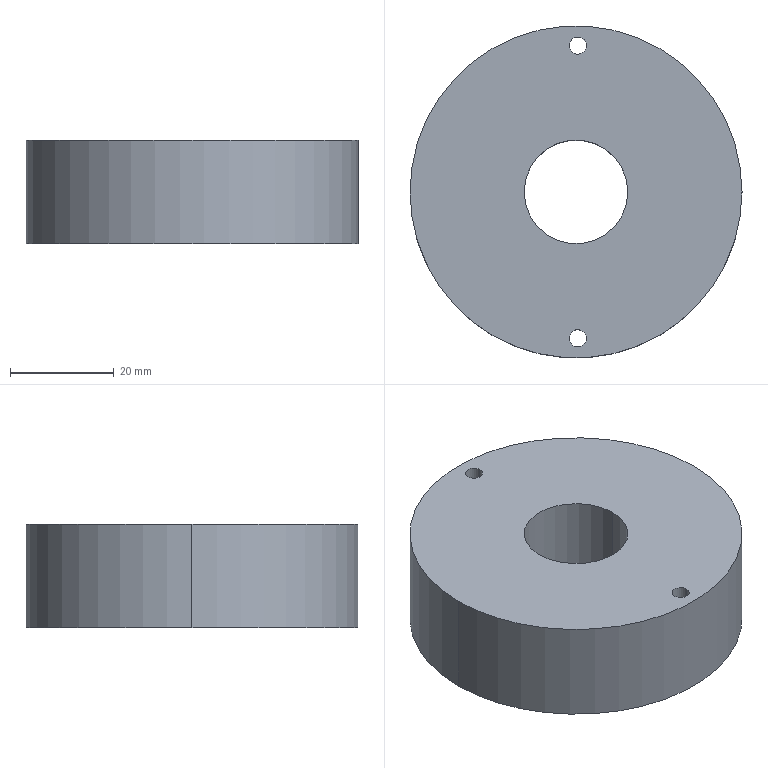Part | SolidWorks | features Extrusion 1, HoleWzd 1 | 1 solid | 10 faces | box 64 x 64 x 20 mm | volume 57715 mm3 | cylinder 8 | plane 2 | commonest cylinder face diameters 3.3 x4 20 x2 64 x2
STEP:
#1=CARTESIAN_POINT('',(-1.65,28.2,20.));
#2=VERTEX_POINT('',#1);
#3=CARTESIAN_POINT('',(1.65,28.2,20.));
#4=VERTEX_POINT('',#3);
#5=CARTESIAN_POINT('',(0.,28.2,20.));
#6=DIRECTION('',(0.,0.,1.));
#7=DIRECTION('',(1.,0.,0.));
#8=AXIS2_PLACEMENT_3D('',#5,#6,#7);
#9=CIRCLE('',#8,1.65);
#10=EDGE_CURVE('',#2,#4,#9,.T.);
#11=ORIENTED_EDGE('',*,*,#10,.T.);
#12=CARTESIAN_POINT('',(1.65,28.2,0.));
#13=VERTEX_POINT('',#12);
#14=CARTESIAN_POINT('',(1.65,28.2,0.));
#15=DIRECTION('',(0.,0.,-1.));
#16=VECTOR('',#15,1000.);
#17=LINE('',#14,#16);
#18=EDGE_CURVE('',#4,#13,#17,.T.);
#19=ORIENTED_EDGE('',*,*,#18,.T.);
#20=CARTESIAN_POINT('',(-1.65,28.2,0.));
#21=VERTEX_POINT('',#20);
#22=CARTESIAN_POINT('',(0.,28.2,0.));
#23=DIRECTION('',(0.,0.,-1.));
#24=DIRECTION('',(-1.,0.,0.));
#25=AXIS2_PLACEMENT_3D('',#22,#23,#24);
#26=CIRCLE('',#25,1.65);
#27=EDGE_CURVE('',#13,#21,#26,.T.);
#28=ORIENTED_EDGE('',*,*,#27,.T.);
#29=CARTESIAN_POINT('',(-1.65,28.2,0.));
#30=DIRECTION('',(0.,0.,-1.));
#31=VECTOR('',#30,1000.);
#32=LINE('',#29,#31);
#33=EDGE_CURVE('',#2,#21,#32,.T.);
#34=ORIENTED_EDGE('',*,*,#33,.F.);
#35=EDGE_LOOP('',(#11,#19,#28,#34));
#36=FACE_OUTER_BOUND('',#35,.T.);
#37=CARTESIAN_POINT('',(0.,28.2,0.));
#38=DIRECTION('',(0.,0.,-1.));
#39=DIRECTION('',(-1.,0.,0.));
#40=AXIS2_PLACEMENT_3D('',#37,#38,#39);
#41=CYLINDRICAL_SURFACE('',#40,1.65);
#42=ADVANCED_FACE('',(#36),#41,.F.);
#43=CARTESIAN_POINT('',(-1.65,-28.2,20.));
#44=VERTEX_POINT('',#43);
#45=CARTESIAN_POINT('',(1.65,-28.2,20.));
#46=VERTEX_POINT('',#45);
#47=CARTESIAN_POINT('',(0.,-28.2,20.));
#48=DIRECTION('',(0.,0.,1.));
#49=DIRECTION('',(1.,0.,0.));
#50=AXIS2_PLACEMENT_3D('',#47,#48,#49);
#51=CIRCLE('',#50,1.65);
#52=EDGE_CURVE('',#44,#46,#51,.T.);
#53=ORIENTED_EDGE('',*,*,#52,.T.);
#54=CARTESIAN_POINT('',(1.65,-28.2,0.));
#55=VERTEX_POINT('',#54);
#56=CARTESIAN_POINT('',(1.65,-28.2,0.));
#57=DIRECTION('',(0.,0.,-1.));
#58=VECTOR('',#57,1000.);
#59=LINE('',#56,#58);
#60=EDGE_CURVE('',#46,#55,#59,.T.);
#61=ORIENTED_EDGE('',*,*,#60,.T.);
#62=CARTESIAN_POINT('',(-1.65,-28.2,0.));
#63=VERTEX_POINT('',#62);
#64=CARTESIAN_POINT('',(0.,-28.2,0.));
#65=DIRECTION('',(0.,0.,-1.));
#66=DIRECTION('',(-1.,0.,0.));
#67=AXIS2_PLACEMENT_3D('',#64,#65,#66);
#68=CIRCLE('',#67,1.65);
#69=EDGE_CURVE('',#55,#63,#68,.T.);
#70=ORIENTED_EDGE('',*,*,#69,.T.);
#71=CARTESIAN_POINT('',(-1.65,-28.2,0.));
#72=DIRECTION('',(0.,0.,-1.));
#73=VECTOR('',#72,1000.);
#74=LINE('',#71,#73);
#75=EDGE_CURVE('',#44,#63,#74,.T.);
#76=ORIENTED_EDGE('',*,*,#75,.F.);
#77=EDGE_LOOP('',(#53,#61,#70,#76));
#78=FACE_OUTER_BOUND('',#77,.T.);
#79=CARTESIAN_POINT('',(0.,-28.2,0.));
#80=DIRECTION('',(0.,0.,-1.));
#81=DIRECTION('',(-1.,0.,0.));
#82=AXIS2_PLACEMENT_3D('',#79,#80,#81);
#83=CYLINDRICAL_SURFACE('',#82,1.65);
#84=ADVANCED_FACE('',(#78),#83,.F.);
#85=CARTESIAN_POINT('',(-10.347,0.,20.));
#86=VERTEX_POINT('',#85);
#87=CARTESIAN_POINT('',(9.653,0.,20.));
#88=VERTEX_POINT('',#87);
#89=CARTESIAN_POINT('',(-0.3472,0.,20.));
#90=DIRECTION('',(0.,0.,1.));
#91=DIRECTION('',(1.,0.,0.));
#92=AXIS2_PLACEMENT_3D('',#89,#90,#91);
#93=CIRCLE('',#92,10.);
#94=EDGE_CURVE('',#86,#88,#93,.T.);
#95=ORIENTED_EDGE('',*,*,#94,.T.);
#96=CARTESIAN_POINT('',(9.653,0.,0.));
#97=VERTEX_POINT('',#96);
#98=CARTESIAN_POINT('',(9.653,0.,20.));
#99=DIRECTION('',(0.,0.,-1.));
#100=VECTOR('',#99,1000.);
#101=LINE('',#98,#100);
#102=EDGE_CURVE('',#88,#97,#101,.T.);
#103=ORIENTED_EDGE('',*,*,#102,.T.);
#104=CARTESIAN_POINT('',(-10.347,0.,0.));
#105=VERTEX_POINT('',#104);
#106=CARTESIAN_POINT('',(-0.3472,0.,0.));
#107=DIRECTION('',(0.,0.,1.));
#108=DIRECTION('',(1.,0.,0.));
#109=AXIS2_PLACEMENT_3D('',#106,#107,#108);
#110=CIRCLE('',#109,10.);
#111=EDGE_CURVE('',#105,#97,#110,.T.);
#112=ORIENTED_EDGE('',*,*,#111,.F.);
#113=CARTESIAN_POINT('',(-10.347,0.,20.));
#114=DIRECTION('',(0.,0.,-1.));
#115=VECTOR('',#114,1000.);
#116=LINE('',#113,#115);
#117=EDGE_CURVE('',#86,#105,#116,.T.);
#118=ORIENTED_EDGE('',*,*,#117,.F.);
#119=EDGE_LOOP('',(#95,#103,#112,#118));
#120=FACE_OUTER_BOUND('',#119,.T.);
#121=CARTESIAN_POINT('',(-0.3472,0.,20.));
#122=DIRECTION('',(0.,0.,-1.));
#123=DIRECTION('',(-1.,0.,0.));
#124=AXIS2_PLACEMENT_3D('',#121,#122,#123);
#125=CYLINDRICAL_SURFACE('',#124,10.);
#126=ADVANCED_FACE('',(#120),#125,.F.);
#127=CARTESIAN_POINT('',(31.653,0.,20.));
#128=VERTEX_POINT('',#127);
#129=CARTESIAN_POINT('',(-32.347,0.,20.));
#130=VERTEX_POINT('',#129);
#131=CARTESIAN_POINT('',(-0.3472,0.,20.));
#132=DIRECTION('',(0.,0.,1.));
#133=DIRECTION('',(1.,0.,0.));
#134=AXIS2_PLACEMENT_3D('',#131,#132,#133);
#135=CIRCLE('',#134,32.);
#136=EDGE_CURVE('',#128,#130,#135,.T.);
#137=ORIENTED_EDGE('',*,*,#136,.F.);
#138=CARTESIAN_POINT('',(31.653,0.,0.));
#139=VERTEX_POINT('',#138);
#140=CARTESIAN_POINT('',(31.653,0.,20.));
#141=DIRECTION('',(0.,0.,-1.));
#142=VECTOR('',#141,1000.);
#143=LINE('',#140,#142);
#144=EDGE_CURVE('',#128,#139,#143,.T.);
#145=ORIENTED_EDGE('',*,*,#144,.T.);
#146=CARTESIAN_POINT('',(-32.347,0.,0.));
#147=VERTEX_POINT('',#146);
#148=CARTESIAN_POINT('',(-0.3472,0.,0.));
#149=DIRECTION('',(0.,0.,1.));
#150=DIRECTION('',(1.,0.,0.));
#151=AXIS2_PLACEMENT_3D('',#148,#149,#150);
#152=CIRCLE('',#151,32.);
#153=EDGE_CURVE('',#139,#147,#152,.T.);
#154=ORIENTED_EDGE('',*,*,#153,.T.);
#155=CARTESIAN_POINT('',(-32.347,0.,20.));
#156=DIRECTION('',(0.,0.,-1.));
#157=VECTOR('',#156,1000.);
#158=LINE('',#155,#157);
#159=EDGE_CURVE('',#130,#147,#158,.T.);
#160=ORIENTED_EDGE('',*,*,#159,.F.);
#161=EDGE_LOOP('',(#137,#145,#154,#160));
#162=FACE_OUTER_BOUND('',#161,.T.);
#163=CARTESIAN_POINT('',(-0.3472,0.,20.));
#164=DIRECTION('',(0.,0.,-1.));
#165=DIRECTION('',(-1.,0.,0.));
#166=AXIS2_PLACEMENT_3D('',#163,#164,#165);
#167=CYLINDRICAL_SURFACE('',#166,32.);
#168=ADVANCED_FACE('',(#162),#167,.T.);
#169=ORIENTED_EDGE('',*,*,#10,.F.);
#170=CARTESIAN_POINT('',(0.,28.2,20.));
#171=DIRECTION('',(0.,0.,1.));
#172=DIRECTION('',(1.,0.,0.));
#173=AXIS2_PLACEMENT_3D('',#170,#171,#172);
#174=CIRCLE('',#173,1.65);
#175=EDGE_CURVE('',#4,#2,#174,.T.);
#176=ORIENTED_EDGE('',*,*,#175,.F.);
#177=EDGE_LOOP('',(#169,#176));
#178=FACE_BOUND('',#177,.T.);
#179=ORIENTED_EDGE('',*,*,#52,.F.);
#180=CARTESIAN_POINT('',(0.,-28.2,20.));
#181=DIRECTION('',(0.,0.,1.));
#182=DIRECTION('',(1.,0.,0.));
#183=AXIS2_PLACEMENT_3D('',#180,#181,#182);
#184=CIRCLE('',#183,1.65);
#185=EDGE_CURVE('',#46,#44,#184,.T.);
#186=ORIENTED_EDGE('',*,*,#185,.F.);
#187=EDGE_LOOP('',(#179,#186));
#188=FACE_BOUND('',#187,.T.);
#189=CARTESIAN_POINT('',(-0.3472,0.,20.));
#190=DIRECTION('',(0.,0.,1.));
#191=DIRECTION('',(1.,0.,0.));
#192=AXIS2_PLACEMENT_3D('',#189,#190,#191);
#193=CIRCLE('',#192,32.);
#194=EDGE_CURVE('',#130,#128,#193,.T.);
#195=ORIENTED_EDGE('',*,*,#194,.T.);
#196=ORIENTED_EDGE('',*,*,#136,.T.);
#197=EDGE_LOOP('',(#195,#196));
#198=FACE_OUTER_BOUND('',#197,.T.);
#199=ORIENTED_EDGE('',*,*,#94,.F.);
#200=CARTESIAN_POINT('',(-0.3472,0.,20.));
#201=DIRECTION('',(0.,0.,1.));
#202=DIRECTION('',(1.,0.,0.));
#203=AXIS2_PLACEMENT_3D('',#200,#201,#202);
#204=CIRCLE('',#203,10.);
#205=EDGE_CURVE('',#88,#86,#204,.T.);
#206=ORIENTED_EDGE('',*,*,#205,.F.);
#207=EDGE_LOOP('',(#199,#206));
#208=FACE_BOUND('',#207,.T.);
#209=CARTESIAN_POINT('',(-0.3472,0.,20.));
#210=DIRECTION('',(0.,0.,1.));
#211=DIRECTION('',(1.,0.,0.));
#212=AXIS2_PLACEMENT_3D('',#209,#210,#211);
#213=PLANE('',#212);
#214=ADVANCED_FACE('',(#178,#188,#198,#208),#213,.T.);
#215=CARTESIAN_POINT('',(0.,28.2,0.));
#216=DIRECTION('',(0.,0.,-1.));
#217=DIRECTION('',(-1.,0.,0.));
#218=AXIS2_PLACEMENT_3D('',#215,#216,#217);
#219=CIRCLE('',#218,1.65);
#220=EDGE_CURVE('',#21,#13,#219,.T.);
#221=ORIENTED_EDGE('',*,*,#220,.F.);
#222=ORIENTED_EDGE('',*,*,#27,.F.);
#223=EDGE_LOOP('',(#221,#222));
#224=FACE_BOUND('',#223,.T.);
#225=CARTESIAN_POINT('',(0.,-28.2,0.));
#226=DIRECTION('',(0.,0.,-1.));
#227=DIRECTION('',(-1.,0.,0.));
#228=AXIS2_PLACEMENT_3D('',#225,#226,#227);
#229=CIRCLE('',#228,1.65);
#230=EDGE_CURVE('',#63,#55,#229,.T.);
#231=ORIENTED_EDGE('',*,*,#230,.F.);
#232=ORIENTED_EDGE('',*,*,#69,.F.);
#233=EDGE_LOOP('',(#231,#232));
#234=FACE_BOUND('',#233,.T.);
#235=CARTESIAN_POINT('',(-0.3472,0.,0.));
#236=DIRECTION('',(0.,0.,1.));
#237=DIRECTION('',(1.,0.,0.));
#238=AXIS2_PLACEMENT_3D('',#235,#236,#237);
#239=CIRCLE('',#238,32.);
#240=EDGE_CURVE('',#147,#139,#239,.T.);
#241=ORIENTED_EDGE('',*,*,#240,.F.);
#242=ORIENTED_EDGE('',*,*,#153,.F.);
#243=EDGE_LOOP('',(#241,#242));
#244=FACE_OUTER_BOUND('',#243,.T.);
#245=ORIENTED_EDGE('',*,*,#111,.T.);
#246=CARTESIAN_POINT('',(-0.3472,0.,0.));
#247=DIRECTION('',(0.,0.,1.));
#248=DIRECTION('',(1.,0.,0.));
#249=AXIS2_PLACEMENT_3D('',#246,#247,#248);
#250=CIRCLE('',#249,10.);
#251=EDGE_CURVE('',#97,#105,#250,.T.);
#252=ORIENTED_EDGE('',*,*,#251,.T.);
#253=EDGE_LOOP('',(#245,#252));
#254=FACE_BOUND('',#253,.T.);
#255=CARTESIAN_POINT('',(-0.3472,0.,0.));
#256=DIRECTION('',(0.,0.,1.));
#257=DIRECTION('',(1.,0.,0.));
#258=AXIS2_PLACEMENT_3D('',#255,#256,#257);
#259=PLANE('',#258);
#260=ADVANCED_FACE('',(#224,#234,#244,#254),#259,.F.);
#261=ORIENTED_EDGE('',*,*,#144,.F.);
#262=ORIENTED_EDGE('',*,*,#194,.F.);
#263=ORIENTED_EDGE('',*,*,#159,.T.);
#264=ORIENTED_EDGE('',*,*,#240,.T.);
#265=EDGE_LOOP('',(#261,#262,#263,#264));
#266=FACE_OUTER_BOUND('',#265,.T.);
#267=CARTESIAN_POINT('',(-0.3472,0.,20.));
#268=DIRECTION('',(0.,0.,-1.));
#269=DIRECTION('',(-1.,0.,0.));
#270=AXIS2_PLACEMENT_3D('',#267,#268,#269);
#271=CYLINDRICAL_SURFACE('',#270,32.);
#272=ADVANCED_FACE('',(#266),#271,.T.);
#273=ORIENTED_EDGE('',*,*,#102,.F.);
#274=ORIENTED_EDGE('',*,*,#205,.T.);
#275=ORIENTED_EDGE('',*,*,#117,.T.);
#276=ORIENTED_EDGE('',*,*,#251,.F.);
#277=EDGE_LOOP('',(#273,#274,#275,#276));
#278=FACE_OUTER_BOUND('',#277,.T.);
#279=CARTESIAN_POINT('',(-0.3472,0.,20.));
#280=DIRECTION('',(0.,0.,-1.));
#281=DIRECTION('',(-1.,0.,0.));
#282=AXIS2_PLACEMENT_3D('',#279,#280,#281);
#283=CYLINDRICAL_SURFACE('',#282,10.);
#284=ADVANCED_FACE('',(#278),#283,.F.);
#285=ORIENTED_EDGE('',*,*,#60,.F.);
#286=ORIENTED_EDGE('',*,*,#185,.T.);
#287=ORIENTED_EDGE('',*,*,#75,.T.);
#288=ORIENTED_EDGE('',*,*,#230,.T.);
#289=EDGE_LOOP('',(#285,#286,#287,#288));
#290=FACE_OUTER_BOUND('',#289,.T.);
#291=CARTESIAN_POINT('',(0.,-28.2,0.));
#292=DIRECTION('',(0.,0.,-1.));
#293=DIRECTION('',(-1.,0.,0.));
#294=AXIS2_PLACEMENT_3D('',#291,#292,#293);
#295=CYLINDRICAL_SURFACE('',#294,1.65);
#296=ADVANCED_FACE('',(#290),#295,.F.);
#297=ORIENTED_EDGE('',*,*,#18,.F.);
#298=ORIENTED_EDGE('',*,*,#175,.T.);
#299=ORIENTED_EDGE('',*,*,#33,.T.);
#300=ORIENTED_EDGE('',*,*,#220,.T.);
#301=EDGE_LOOP('',(#297,#298,#299,#300));
#302=FACE_OUTER_BOUND('',#301,.T.);
#303=CARTESIAN_POINT('',(0.,28.2,0.));
#304=DIRECTION('',(0.,0.,-1.));
#305=DIRECTION('',(-1.,0.,0.));
#306=AXIS2_PLACEMENT_3D('',#303,#304,#305);
#307=CYLINDRICAL_SURFACE('',#306,1.65);
#308=ADVANCED_FACE('',(#302),#307,.F.);
#309=CLOSED_SHELL('',(#42,#84,#126,#168,#214,#260,#272,#284,#296,#308));
#310=MANIFOLD_SOLID_BREP('',#309);
#311=CARTESIAN_POINT('',(0.,0.,0.));
#312=DIRECTION('',(0.,0.,1.));
#313=DIRECTION('',(1.,0.,0.));
#314=AXIS2_PLACEMENT_3D('',#311,#312,#313);
#315=(LENGTH_UNIT()NAMED_UNIT(*)SI_UNIT(.MILLI.,.METRE.));
#316=UNCERTAINTY_MEASURE_WITH_UNIT(LENGTH_MEASURE(0.00001),#315,'','');
#317=(NAMED_UNIT(*)PLANE_ANGLE_UNIT()SI_UNIT($,.RADIAN.));
#318=(NAMED_UNIT(*)SI_UNIT($,.STERADIAN.)SOLID_ANGLE_UNIT());
#319=(GEOMETRIC_REPRESENTATION_CONTEXT(3)GLOBAL_UNCERTAINTY_ASSIGNED_CONTEXT((#316))GLOBAL_UNIT_ASSIGNED_CONTEXT((#315,#317,#318))REPRESENTATION_CONTEXT('',''));
#320=ADVANCED_BREP_SHAPE_REPRESENTATION('',(#310,#314),#319);